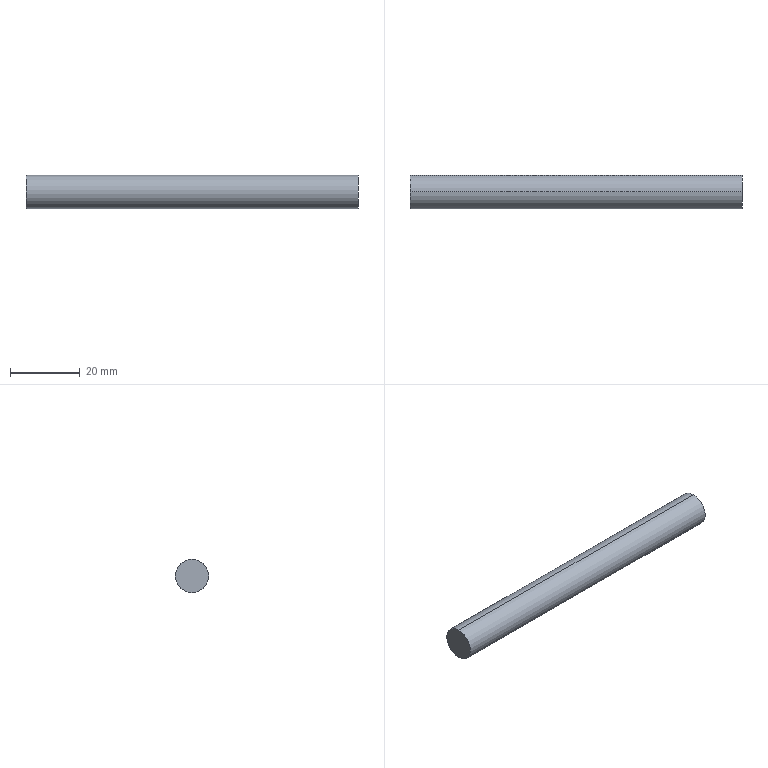Part | STEP file | 4-20.sldasm-Part-108 | 1 solid | 4 faces | box 95 x 9.525 x 9.525 mm | volume 6769 mm3 | cylinder 2 | plane 2 | commonest cylinder face diameters 9.525 x2
STEP:
#1=CARTESIAN_POINT('',(143.125,85.,48.763));
#2=VERTEX_POINT('',#1);
#3=CARTESIAN_POINT('',(143.125,85.,39.237));
#4=VERTEX_POINT('',#3);
#5=CARTESIAN_POINT('',(143.125,85.,44.));
#6=DIRECTION('',(-1.,0.,0.));
#7=DIRECTION('',(0.,0.,-1.));
#8=AXIS2_PLACEMENT_3D('',#5,#6,#7);
#9=CIRCLE('',#8,4.763);
#10=EDGE_CURVE('',#2,#4,#9,.T.);
#11=ORIENTED_EDGE('',*,*,#10,.F.);
#12=CARTESIAN_POINT('',(238.125,85.,48.763));
#13=VERTEX_POINT('',#12);
#14=CARTESIAN_POINT('',(-431.8,85.,48.763));
#15=DIRECTION('',(1.,0.,0.));
#16=VECTOR('',#15,1000.);
#17=LINE('',#14,#16);
#18=EDGE_CURVE('',#2,#13,#17,.T.);
#19=ORIENTED_EDGE('',*,*,#18,.T.);
#20=CARTESIAN_POINT('',(238.125,85.,39.237));
#21=VERTEX_POINT('',#20);
#22=CARTESIAN_POINT('',(238.125,85.,44.));
#23=DIRECTION('',(1.,0.,0.));
#24=DIRECTION('',(0.,0.,1.));
#25=AXIS2_PLACEMENT_3D('',#22,#23,#24);
#26=CIRCLE('',#25,4.763);
#27=EDGE_CURVE('',#21,#13,#26,.T.);
#28=ORIENTED_EDGE('',*,*,#27,.F.);
#29=CARTESIAN_POINT('',(-431.8,85.,39.237));
#30=DIRECTION('',(1.,0.,0.));
#31=VECTOR('',#30,1000.);
#32=LINE('',#29,#31);
#33=EDGE_CURVE('',#4,#21,#32,.T.);
#34=ORIENTED_EDGE('',*,*,#33,.F.);
#35=EDGE_LOOP('',(#11,#19,#28,#34));
#36=FACE_OUTER_BOUND('',#35,.T.);
#37=CARTESIAN_POINT('',(-431.8,85.,44.));
#38=DIRECTION('',(1.,0.,0.));
#39=DIRECTION('',(0.,0.,-1.));
#40=AXIS2_PLACEMENT_3D('',#37,#38,#39);
#41=CYLINDRICAL_SURFACE('',#40,4.763);
#42=ADVANCED_FACE('',(#36),#41,.T.);
#43=ORIENTED_EDGE('',*,*,#27,.T.);
#44=CARTESIAN_POINT('',(238.125,85.,44.));
#45=DIRECTION('',(1.,0.,0.));
#46=DIRECTION('',(0.,0.,1.));
#47=AXIS2_PLACEMENT_3D('',#44,#45,#46);
#48=CIRCLE('',#47,4.763);
#49=EDGE_CURVE('',#13,#21,#48,.T.);
#50=ORIENTED_EDGE('',*,*,#49,.T.);
#51=EDGE_LOOP('',(#43,#50));
#52=FACE_OUTER_BOUND('',#51,.T.);
#53=CARTESIAN_POINT('',(238.125,-302.,90.));
#54=DIRECTION('',(-1.,0.,0.));
#55=DIRECTION('',(0.,0.,1.));
#56=AXIS2_PLACEMENT_3D('',#53,#54,#55);
#57=PLANE('',#56);
#58=ADVANCED_FACE('',(#52),#57,.F.);
#59=ORIENTED_EDGE('',*,*,#18,.F.);
#60=CARTESIAN_POINT('',(143.125,85.,44.));
#61=DIRECTION('',(-1.,0.,0.));
#62=DIRECTION('',(0.,0.,-1.));
#63=AXIS2_PLACEMENT_3D('',#60,#61,#62);
#64=CIRCLE('',#63,4.763);
#65=EDGE_CURVE('',#4,#2,#64,.T.);
#66=ORIENTED_EDGE('',*,*,#65,.F.);
#67=ORIENTED_EDGE('',*,*,#33,.T.);
#68=ORIENTED_EDGE('',*,*,#49,.F.);
#69=EDGE_LOOP('',(#59,#66,#67,#68));
#70=FACE_OUTER_BOUND('',#69,.T.);
#71=CARTESIAN_POINT('',(-431.8,85.,44.));
#72=DIRECTION('',(1.,0.,0.));
#73=DIRECTION('',(0.,0.,-1.));
#74=AXIS2_PLACEMENT_3D('',#71,#72,#73);
#75=CYLINDRICAL_SURFACE('',#74,4.763);
#76=ADVANCED_FACE('',(#70),#75,.T.);
#77=ORIENTED_EDGE('',*,*,#65,.T.);
#78=ORIENTED_EDGE('',*,*,#10,.T.);
#79=EDGE_LOOP('',(#77,#78));
#80=FACE_OUTER_BOUND('',#79,.T.);
#81=CARTESIAN_POINT('',(143.125,529.8,44.));
#82=DIRECTION('',(1.,0.,0.));
#83=DIRECTION('',(0.,0.,-1.));
#84=AXIS2_PLACEMENT_3D('',#81,#82,#83);
#85=PLANE('',#84);
#86=ADVANCED_FACE('',(#80),#85,.F.);
#87=CLOSED_SHELL('',(#42,#58,#76,#86));
#88=MANIFOLD_SOLID_BREP('',#87);
#89=CARTESIAN_POINT('',(0.,0.,0.));
#90=DIRECTION('',(0.,0.,1.));
#91=DIRECTION('',(1.,0.,0.));
#92=AXIS2_PLACEMENT_3D('',#89,#90,#91);
#93=(LENGTH_UNIT()NAMED_UNIT(*)SI_UNIT(.MILLI.,.METRE.));
#94=UNCERTAINTY_MEASURE_WITH_UNIT(LENGTH_MEASURE(0.00001),#93,'','');
#95=(NAMED_UNIT(*)PLANE_ANGLE_UNIT()SI_UNIT($,.RADIAN.));
#96=(NAMED_UNIT(*)SI_UNIT($,.STERADIAN.)SOLID_ANGLE_UNIT());
#97=(GEOMETRIC_REPRESENTATION_CONTEXT(3)GLOBAL_UNCERTAINTY_ASSIGNED_CONTEXT((#94))GLOBAL_UNIT_ASSIGNED_CONTEXT((#93,#95,#96))REPRESENTATION_CONTEXT('',''));
#98=ADVANCED_BREP_SHAPE_REPRESENTATION('',(#88,#92),#97);